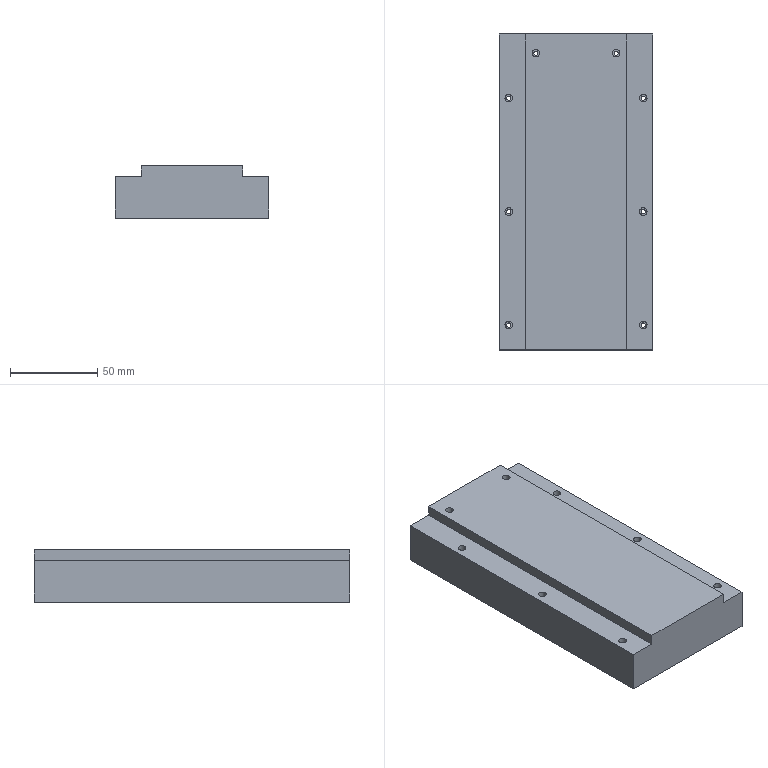NC program | NX | posted with a generic post | part box 88 x 181.05 x 30 mm
Lines 5692 to 6442 of 14572:
(CURVE_DRIVE_3_COPY , TOOL : BALL_END_R1-4-D4-50)
N11304 T14 M6
N11306 G54
N11308 G3P2 X0. Y0. Z0. I90. J12.8666 K-83.5258
N11310 G53.1
N11312 G17 G43 G0 G90 X-24.469 Y-28.966 Z32.437 S6500 H14 M3
N11314 Z2.912
N11316 G94 G1 Z1.229 F2000.
N11318 X-24.473 Z0.76
N11320 X-24.621 Y-28.979 Z0.314
N11322 X-24.898 Y-29.002 Z-0.063
N11324 X-25.279 Y-29.035 Z-0.336
N11326 X-25.725 Y-29.073 Z-0.478
N11328 X-25.965 Y-29.093 Z-0.514
N11330 X-26.205 Y-29.113 Z-0.51
N11332 X-26.462 Y-29.135 Z-0.502
N11334 X-26.833 Y-29.167 Z-0.441
N11336 X-26.956 Y-29.158
N11338 X-27.058 Y-29.143 Z-0.433
N11340 X-26.954 Y-29.134 Z-0.462
N11342 X-26.457 Y-29.092 Z-0.544
N11344 X-26.264 Y-29.075 Z-0.551
N11346 X-25.96 Y-29.05 Z-0.555
N11348 X-25.488 Y-29.009 Z-0.487
N11350 X-25.377 Y-28.961 Z-0.492
N11352 X-25.506 Y-28.972 Z-0.53
N11354 X-25.958 Y-29.01 Z-0.592
N11356 X-26.452 Y-29.052 Z-0.582
N11358 X-26.949 Y-29.095 Z-0.5
N11360 X-27.209 Y-29.117 Z-0.424
N11362 X-27.347 Y-29.087 Z-0.422
N11364 X-26.944 Y-29.052 Z-0.54
N11366 X-26.447 Y-29.01 Z-0.624
N11368 X-25.95 Y-28.968 Z-0.634
N11370 X-25.521 Y-28.931 Z-0.575
N11372 X-25.454 Y-28.926 Z-0.558
N11374 X-25.262 Y-28.909 Z-0.497
N11376 X-25.148 Y-28.858 Z-0.502
N11378 X-25.449 Y-28.884 Z-0.599
N11380 X-25.536 Y-28.891 Z-0.62
N11382 X-25.946 Y-28.926 Z-0.675
N11384 X-25.987 Y-28.929 Z-0.678
N11386 X-26.443 Y-28.968 Z-0.665
N11388 X-26.94 Y-29.01 Z-0.58
N11390 X-27.477 Y-29.056 Z-0.419
N11392 X-27.602 Y-29.025 Z-0.414
N11394 X-27.432 Y-29.01 Z-0.471
N11396 X-26.935 Y-28.968 Z-0.62
N11398 X-26.419 Y-28.924 Z-0.708
N11400 X-26.002 Y-28.889 Z-0.72
N11402 X-25.866 Y-28.877 Z-0.709
N11404 X-25.55 Y-28.85 Z-0.665
N11406 X-25.444 Y-28.841 Z-0.639
N11408 X-25.047 Y-28.808 Z-0.512
N11410 X-24.961 Y-28.76 Z-0.516
N11412 X-25.048 Y-28.768 Z-0.553
N11414 X-25.439 Y-28.801 Z-0.677
N11416 X-25.565 Y-28.812 Z-0.709
N11418 X-25.839 Y-28.835 Z-0.747
N11420 X-26.016 Y-28.85 Z-0.761
N11422 X-26.391 Y-28.882 Z-0.75
N11424 X-26.468 Y-28.888 Z-0.741
N11426 X-26.93 Y-28.928 Z-0.659
N11428 X-27.427 Y-28.97 Z-0.507
N11430 X-27.708 Y-28.994 Z-0.413
N11432 X-27.809 Y-28.962
N11434 X-27.422 Y-28.929 Z-0.545
N11436 X-26.916 Y-28.886 Z-0.701
N11438 X-26.429 Y-28.844 Z-0.787
N11440 X-26.363 Y-28.839 Z-0.793
N11442 X-26.031 Y-28.81 Z-0.803
N11444 X-25.81 Y-28.792 Z-0.785
N11446 X-25.579 Y-28.772 Z-0.753
N11448 X-25.435 Y-28.76 Z-0.717
N11450 X-25.079 Y-28.729 Z-0.604
N11452 X-24.882 Y-28.713 Z-0.517
N11454 X-24.802 Y-28.664 Z-0.518
N11456 X-24.933 Y-28.675 Z-0.581
N11458 X-25.11 Y-28.69 Z-0.656
N11460 X-25.43 Y-28.717 Z-0.757
N11462 X-25.594 Y-28.731 Z-0.798
N11464 X-25.782 Y-28.747 Z-0.824
N11466 X-26.046 Y-28.77 Z-0.846
N11468 X-26.334 Y-28.794 Z-0.837
N11470 X-26.497 Y-28.808 Z-0.817
N11472 X-26.886 Y-28.841 Z-0.748
N11474 X-27.418 Y-28.887 Z-0.583
N11476 X-27.911 Y-28.929 Z-0.413
N11478 X-28.013 Y-28.895
N11480 X-27.406 Y-28.844 Z-0.623
N11482 X-26.858 Y-28.797 Z-0.794
N11484 X-26.419 Y-28.76 Z-0.87
N11486 X-26.305 Y-28.75 Z-0.881
N11488 X-26.06 Y-28.729 Z-0.889
N11490 X-25.753 Y-28.703 Z-0.863
N11492 X-25.609 Y-28.691 Z-0.843
N11494 X-25.425 Y-28.675 Z-0.797
N11496 X-25.141 Y-28.651 Z-0.708
N11498 X-24.934 Y-28.634 Z-0.621
N11500 X-24.722 Y-28.616 Z-0.518
N11502 X-24.659 Y-28.568 Z-0.519
N11504 X-24.72 Y-28.574 Z-0.556
N11506 X-24.965 Y-28.594 Z-0.674
N11508 X-25.173 Y-28.612 Z-0.76
N11510 X-25.423 Y-28.633 Z-0.838
N11512 X-25.624 Y-28.65 Z-0.888
N11514 X-25.724 Y-28.659 Z-0.902
N11516 X-26.075 Y-28.689 Z-0.931
N11518 X-26.276 Y-28.706 Z-0.925
N11520 X-26.414 Y-28.718 Z-0.912
N11522 X-26.829 Y-28.753 Z-0.84
N11524 X-26.911 Y-28.76 Z-0.818
N11526 X-27.347 Y-28.797 Z-0.68
N11528 X-28.115 Y-28.862 Z-0.412
N11530 X-28.217 Y-28.829
N11532 X-27.289 Y-28.75 Z-0.737
N11534 X-26.906 Y-28.718 Z-0.858
N11536 X-26.8 Y-28.709 Z-0.887
N11538 X-26.409 Y-28.676 Z-0.954
N11540 X-26.248 Y-28.662 Z-0.969
N11542 X-26.09 Y-28.648 Z-0.974
N11544 X-25.695 Y-28.615 Z-0.941
N11546 X-25.638 Y-28.61 Z-0.933
N11548 X-25.416 Y-28.591 Z-0.878
N11550 X-25.187 Y-28.572 Z-0.807
N11552 X-24.919 Y-28.549 Z-0.692
N11554 X-24.735 Y-28.533 Z-0.603
N11556 X-24.601 Y-28.522 Z-0.522
N11558 X-24.546 Y-28.475 Z-0.526
N11560 X-24.75 Y-28.493 Z-0.649
N11562 X-25.028 Y-28.516 Z-0.781
N11564 X-25.235 Y-28.534 Z-0.865
N11566 X-25.411 Y-28.549 Z-0.919
N11568 X-25.666 Y-28.571 Z-0.98
N11570 X-26.105 Y-28.608 Z-1.017
N11572 X-26.219 Y-28.618 Z-1.013
N11574 X-26.405 Y-28.633 Z-0.995
N11576 X-26.771 Y-28.664 Z-0.933
N11578 X-26.902 Y-28.676 Z-0.898
N11580 X-27.23 Y-28.704 Z-0.794
N11582 X-28.32 Y-28.796 Z-0.412
N11584 X-28.424 Y-28.763
N11586 X-28.282 Y-28.751 Z-0.459
N11588 X-27.171 Y-28.657 Z-0.851
N11590 X-26.897 Y-28.633 Z-0.938
N11592 X-26.742 Y-28.62 Z-0.98
N11594 X-26.4 Y-28.591 Z-1.037
N11596 X-26.19 Y-28.573 Z-1.057
N11598 X-26.12 Y-28.567 Z-1.06
N11600 X-25.668 Y-28.529 Z-1.023
N11602 X-25.406 Y-28.507 Z-0.961
N11604 X-25.217 Y-28.49 Z-0.9
N11606 X-25.059 Y-28.477 Z-0.835
N11608 X-24.765 Y-28.452 Z-0.696
N11610 X-24.492 Y-28.429 Z-0.531
N11612 X-24.441 Y-28.383 Z-0.534
N11614 X-24.78 Y-28.412 Z-0.741
N11616 X-25.09 Y-28.438 Z-0.888
N11618 X-25.297 Y-28.456 Z-0.97
N11620 X-25.401 Y-28.465 Z-1.002
N11622 X-25.683 Y-28.489 Z-1.068
N11624 X-26.134 Y-28.527 Z-1.102
N11626 X-26.395 Y-28.549 Z-1.078
N11628 X-26.714 Y-28.576 Z-1.026
N11630 X-26.892 Y-28.592 Z-0.978
N11632 X-27.113 Y-28.61 Z-0.908
N11634 X-28.523 Y-28.73 Z-0.411
N11636 X-28.625 Y-28.698
N11638 X-27.054 Y-28.564 Z-0.964
N11640 X-26.887 Y-28.55 Z-1.017
N11642 X-26.685 Y-28.533 Z-1.072
N11644 X-26.39 Y-28.508 Z-1.12
N11646 X-26.133 Y-28.486 Z-1.144
N11648 X-25.741 Y-28.452 Z-1.116
N11650 X-25.645 Y-28.444 Z-1.103
N11652 X-25.397 Y-28.423 Z-1.043
N11654 X-25.246 Y-28.41 Z-0.992
N11656 X-25.121 Y-28.4 Z-0.94
N11658 X-24.794 Y-28.372 Z-0.787
N11660 X-24.569 Y-28.353 Z-0.652
N11662 X-24.391 Y-28.337 Z-0.536
N11664 X-24.343 Y-28.292 Z-0.537
N11666 X-24.625 Y-28.316 Z-0.723
N11668 X-24.809 Y-28.332 Z-0.833
N11670 X-25.151 Y-28.361 Z-0.993
N11672 X-25.358 Y-28.378 Z-1.074
N11674 X-25.64 Y-28.402 Z-1.144
N11676 X-25.772 Y-28.414 Z-1.162
N11678 X-26.137 Y-28.445 Z-1.186
N11680 X-26.43 Y-28.47 Z-1.154
N11682 X-26.657 Y-28.489 Z-1.118
N11684 X-26.883 Y-28.508 Z-1.057
N11686 X-26.996 Y-28.518 Z-1.021
N11688 X-28.727 Y-28.665 Z-0.411
N11690 X-28.83 Y-28.632 Z-0.412
N11692 X-26.878 Y-28.466 Z-1.096
N11694 X-26.629 Y-28.445 Z-1.164
N11696 X-26.381 Y-28.424 Z-1.204
N11698 X-26.132 Y-28.403 Z-1.228
N11700 X-25.803 Y-28.375 Z-1.208
N11702 X-25.727 Y-28.368 Z-1.201
N11704 X-25.635 Y-28.36 Z-1.185
N11706 X-25.389 Y-28.34 Z-1.127
N11708 X-25.182 Y-28.322 Z-1.046
N11710 X-24.824 Y-28.291 Z-0.879
N11712 X-24.682 Y-28.279 Z-0.794
N11714 X-24.393 Y-28.255 Z-0.607
N11716 X-24.294 Y-28.246 Z-0.539
N11718 X-24.247 Y-28.201
N11720 X-24.388 Y-28.213 Z-0.639
N11722 X-24.738 Y-28.243 Z-0.865
N11724 X-24.838 Y-28.251 Z-0.925
N11726 X-25.213 Y-28.283 Z-1.099
N11728 X-25.382 Y-28.297 Z-1.165
N11730 X-25.631 Y-28.319 Z-1.226
N11732 X-25.742 Y-28.328 Z-1.245
N11734 X-25.947 Y-28.346 Z-1.262
N11736 X-26.128 Y-28.361 Z-1.27
N11738 X-26.376 Y-28.382 Z-1.247
N11740 X-26.6 Y-28.401 Z-1.211
N11742 X-26.879 Y-28.425 Z-1.134
N11744 X-28.932 Y-28.599 Z-0.411
N11746 X-29.033 Y-28.567
N11748 X-26.868 Y-28.382 Z-1.175
N11750 X-26.571 Y-28.357 Z-1.258
N11752 X-26.371 Y-28.34 Z-1.29
N11754 X-26.123 Y-28.319 Z-1.312
N11756 X-25.874 Y-28.298 Z-1.301
N11758 X-25.756 Y-28.288 Z-1.29
N11760 X-25.626 Y-28.277 Z-1.267
N11762 X-25.451 Y-28.262 Z-1.226
N11764 X-25.378 Y-28.256 Z-1.204
N11766 X-25.244 Y-28.244 Z-1.152
N11768 X-24.853 Y-28.211 Z-0.971
N11770 X-24.416 Y-28.174 Z-0.694
N11772 X-24.202 Y-28.156 Z-0.541
N11774 X-24.163 Y-28.111
N11776 X-24.191 Y-28.113 Z-0.565
N11778 X-24.379 Y-28.129 Z-0.698
N11780 X-24.448 Y-28.135 Z-0.751
N11782 X-24.868 Y-28.171 Z-1.018
N11784 X-25.32 Y-28.209 Z-1.224
N11786 X-25.373 Y-28.214 Z-1.243
N11788 X-25.482 Y-28.223 Z-1.275
N11790 X-25.621 Y-28.235 Z-1.308
N11792 X-25.771 Y-28.248 Z-1.334
N11794 X-25.87 Y-28.256 Z-1.344
N11796 X-26.118 Y-28.277 Z-1.355
N11798 X-26.367 Y-28.298 Z-1.333
N11800 X-26.542 Y-28.313 Z-1.304
N11802 X-26.864 Y-28.34 Z-1.214
N11804 X-29.137 Y-28.534 Z-0.412
N11806 X-29.241 Y-28.501 Z-0.413
N11808 X-29.163 Y-28.494 Z-0.437
N11810 X-26.859 Y-28.298 Z-1.253
N11812 X-26.514 Y-28.269 Z-1.351
N11814 X-26.362 Y-28.256 Z-1.376
N11816 X-26.113 Y-28.235 Z-1.397
N11818 X-25.865 Y-28.214 Z-1.387
N11820 X-25.786 Y-28.207 Z-1.379
N11822 X-25.616 Y-28.193 Z-1.35
N11824 X-25.513 Y-28.184 Z-1.325
N11826 X-25.334 Y-28.169 Z-1.27
N11828 X-24.883 Y-28.13 Z-1.064
N11830 X-24.479 Y-28.096 Z-0.808
N11832 X-24.374 Y-28.087 Z-0.728
N11834 X-24.205 Y-28.073 Z-0.609
N11836 X-24.127 Y-28.066 Z-0.54
N11838 X-24.091 Y-28.021 Z-0.538
N11840 X-24.22 Y-28.032 Z-0.652
N11842 X-24.369 Y-28.045 Z-0.758
N11844 X-24.51 Y-28.057 Z-0.866
N11846 X-24.898 Y-28.09 Z-1.111
N11848 X-25.363 Y-28.13 Z-1.322
N11850 X-25.544 Y-28.145 Z-1.375
N11852 X-25.612 Y-28.151 Z-1.391
N11854 X-25.801 Y-28.167 Z-1.424
N11856 X-25.933 Y-28.178 Z-1.433
N11858 X-26.109 Y-28.193 Z-1.439
N11860 X-26.357 Y-28.214 Z-1.419
N11862 X-26.485 Y-28.225 Z-1.398
N11864 X-26.854 Y-28.256 Z-1.292
N11866 X-28.648 Y-28.409 Z-0.654
N11868 X-29.22 Y-28.458 Z-0.453
N11870 X-29.346 Y-28.468 Z-0.414
N11872 X-29.447 Y-28.435 Z-0.413
N11874 X-29.276 Y-28.421 Z-0.469
N11876 X-27.346 Y-28.257 Z-1.153
N11878 X-26.849 Y-28.214 Z-1.332
N11880 X-26.456 Y-28.181 Z-1.445
N11882 X-26.352 Y-28.172 Z-1.462
N11884 X-26.104 Y-28.151 Z-1.482
N11886 X-25.816 Y-28.126 Z-1.468
N11888 X-25.575 Y-28.106 Z-1.425
N11890 X-25.352 Y-28.087 Z-1.358
N11892 X-24.912 Y-28.05 Z-1.158
N11894 X-24.541 Y-28.018 Z-0.923
N11896 X-24.365 Y-28.003 Z-0.787
N11898 X-24.235 Y-27.992 Z-0.696
N11900 X-24.056 Y-27.977 Z-0.538
N11902 X-24.023 Y-27.933 Z-0.539
N11904 X-24.25 Y-27.952 Z-0.739
N11906 X-24.36 Y-27.961 Z-0.816
N11908 X-24.572 Y-27.979 Z-0.98
N11910 X-24.927 Y-28.01 Z-1.205
N11912 X-25.354 Y-28.046 Z-1.401
N11914 X-25.432 Y-28.052 Z-1.427
N11916 X-25.613 Y-28.068 Z-1.475
N11918 X-25.851 Y-28.088 Z-1.514
N11920 X-26.099 Y-28.109 Z-1.523
N11922 X-26.348 Y-28.13 Z-1.505
N11924 X-26.428 Y-28.137 Z-1.492
N11926 X-26.529 Y-28.146 Z-1.464
N11928 X-26.606 Y-28.152 Z-1.447
N11930 X-26.851 Y-28.173 Z-1.368
N11932 X-27.469 Y-28.226 Z-1.144
N11934 X-29.546 Y-28.402 Z-0.412
N11936 X-29.64 Y-28.372 Z-0.411
N11938 X-27.498 Y-28.189 Z-1.167
N11940 X-26.877 Y-28.136 Z-1.395
N11942 X-26.857 Y-28.135 Z-1.404
N11944 X-26.946 Y-28.105 Z-1.402
N11946 X-27.526 Y-28.154 Z-1.19
N11948 X-29.731 Y-28.342 Z-0.41
N11950 X-29.824 Y-28.312
N11952 X-27.555 Y-28.119 Z-1.213
N11954 X-27.038 Y-28.075 Z-1.402
N11956 X-27.137 Y-28.042 Z-1.403
N11958 X-27.585 Y-28.081 Z-1.237
N11960 X-29.927 Y-28.28 Z-0.411
N11962 X-30.035 Y-28.246 Z-0.413
N11964 X-29.803 Y-28.226 Z-0.491
N11966 X-27.618 Y-28.04 Z-1.263
N11968 X-27.24 Y-28.008 Z-1.404
N11970 X-27.343 Y-27.974
N11972 X-27.65 Y-28. Z-1.29
N11974 X-29.798 Y-28.183 Z-0.53
N11976 X-30.143 Y-28.212 Z-0.413
N11978 X-30.248 Y-28.178
N11980 X-29.793 Y-28.139 Z-0.569
N11982 X-27.682 Y-27.96 Z-1.316
N11984 X-27.444 Y-27.94 Z-1.404
N11986 X-27.547 Y-27.905
N11988 X-28.233 Y-27.964 Z-1.158
N11990 X-29.814 Y-28.098 Z-0.6
N11992 X-30.353 Y-28.144 Z-0.413
N11994 X-30.46 Y-28.109 Z-0.412
N11996 X-28.303 Y-27.926 Z-1.171
N11998 X-27.653 Y-27.87 Z-1.403
N12000 X-27.753 Y-27.838
N12002 X-30.561 Y-28.076 Z-0.412
N12004 X-30.667 Y-28.042 Z-0.411
N12006 X-27.861 Y-27.803 Z-1.403
N12008 X-27.972 Y-27.769 Z-1.404
N12010 X-28.144 Y-27.783 Z-1.34
N12012 X-30.722 Y-28.003 Z-0.429
N12014 X-30.777 Y-28.007 Z-0.412
N12016 X-30.886 Y-27.971 Z-0.411
N12018 X-28.297 Y-27.751 Z-1.326
N12020 X-28.086 Y-27.733 Z-1.405
N12022 X-28.199 Y-27.698 Z-1.406
N12024 X-28.599 Y-27.732 Z-1.258
N12026 X-30.997 Y-27.936 Z-0.411
N12028 X-31.108 Y-27.9
N12030 X-28.715 Y-27.696 Z-1.258
N12032 X-28.311 Y-27.662 Z-1.407
N12034 X-28.424 Y-27.627 Z-1.408
N12036 X-28.839 Y-27.662 Z-1.251
N12038 X-31.219 Y-27.865 Z-0.411
N12040 X-31.329 Y-27.829
N12042 X-28.749 Y-27.61 Z-1.323
N12044 X-28.533 Y-27.591 Z-1.407
N12046 X-28.639 Y-27.555 Z-1.405
N12048 X-28.962 Y-27.583 Z-1.286
N12050 X-31.44 Y-27.794 Z-0.411
N12052 X-31.551 Y-27.759 Z-0.412
N12054 X-29.022 Y-27.544 Z-1.303
N12056 X-28.743 Y-27.52 Z-1.403
N12058 X-28.85 Y-27.486
N12060 X-31.563 Y-27.716 Z-0.443
N12062 X-31.66 Y-27.725 Z-0.413
N12064 X-31.767 Y-27.69
N12066 X-31.622 Y-27.678 Z-0.459
N12068 X-28.956 Y-27.451 Z-1.403
N12070 X-29.069 Y-27.417 Z-1.404
N12072 X-29.269 Y-27.434 Z-1.33
N12074 X-31.705 Y-27.641 Z-0.469
N12076 X-31.873 Y-27.655 Z-0.412
N12078 X-31.98 Y-27.62 Z-0.411
N12080 X-29.863 Y-27.44 Z-1.158
N12082 X-29.713 Y-27.427 Z-1.214
N12084 X-29.24 Y-27.387 Z-1.381
N12086 X-29.181 Y-27.382 Z-1.405
N12088 X-29.29 Y-27.346 Z-1.404
N12090 X-30.526 Y-27.451 Z-0.963
N12092 X-32.09 Y-27.584 Z-0.41
N12094 X-32.203 Y-27.548
N12096 X-29.931 Y-27.354 Z-1.214
N12098 X-29.702 Y-27.335 Z-1.299
N12100 X-29.401 Y-27.309 Z-1.404
N12102 X-29.512 Y-27.274 Z-1.405
N12104 X-30.518 Y-27.36 Z-1.045
N12106 X-32.316 Y-27.513 Z-0.411
N12108 X-32.426 Y-27.478 Z-0.413
N12110 X-32.177 Y-27.457 Z-0.496
N12112 X-29.997 Y-27.272 Z-1.267
N12114 X-29.622 Y-27.24 Z-1.405
N12116 X-29.728 Y-27.206
N12118 X-30.029 Y-27.231 Z-1.293
N12120 X-32.172 Y-27.414 Z-0.535
N12122 X-32.533 Y-27.444 Z-0.413
N12124 X-32.639 Y-27.41
N12126 X-31.64 Y-27.325 Z-0.761
N12128 X-30.061 Y-27.191 Z-1.32
N12130 X-29.833 Y-27.171 Z-1.405
N12132 X-29.939 Y-27.136 Z-1.404
N12134 X-31.133 Y-27.238 Z-0.979
N12136 X-32.172 Y-27.326 Z-0.611
N12138 X-32.746 Y-27.375 Z-0.412
N12140 X-32.854 Y-27.34
N12142 X-30.694 Y-27.156 Z-1.173
N12144 X-30.046 Y-27.101 Z-1.403
N12146 X-30.154 Y-27.066 Z-1.402
N12148 X-32.963 Y-27.305 Z-0.411
N12150 X-33.073 Y-27.269 Z-0.412
N12152 X-30.267 Y-27.031 Z-1.403
N12154 X-30.379 Y-26.996 Z-1.405
N12156 X-30.592 Y-27.014 Z-1.325
N12158 X-33.135 Y-27.23 Z-0.427
N12160 X-33.183 Y-27.234 Z-0.412
N12162 X-33.292 Y-27.198 Z-0.411
N12164 X-30.645 Y-26.973 Z-1.348
N12166 X-30.493 Y-26.96 Z-1.406
N12168 X-30.606 Y-26.924
N12170 X-31.048 Y-26.962 Z-1.243
N12172 X-33.404 Y-27.162 Z-0.411
N12174 X-33.516 Y-27.127
N12176 X-31.132 Y-26.924 Z-1.252
N12178 X-30.718 Y-26.889 Z-1.407
N12180 X-30.83 Y-26.854 Z-1.408
N12182 X-31.234 Y-26.888 Z-1.255
N12184 X-33.626 Y-27.092 Z-0.411
N12186 X-33.736 Y-27.056
N12188 X-31.122 Y-26.834 Z-1.335
N12190 X-30.937 Y-26.818 Z-1.406
N12192 X-31.043 Y-26.782 Z-1.404
N12194 X-31.848 Y-26.851 Z-1.116
N12196 X-33.847 Y-27.021 Z-0.411
N12198 X-33.958 Y-26.986 Z-0.412
N12200 X-32.602 Y-26.871 Z-0.888
N12202 X-31.148 Y-26.747 Z-1.403
N12204 X-31.254 Y-26.713
N12206 X-33.957 Y-26.943 Z-0.447
N12208 X-34.066 Y-26.952 Z-0.413
N12210 X-34.172 Y-26.917
N12212 X-34.016 Y-26.904 Z-0.463
N12214 X-31.362 Y-26.678 Z-1.403
N12216 X-31.477 Y-26.644 Z-1.405
N12218 X-31.595 Y-26.654 Z-1.358
N12220 X-34.078 Y-26.865 Z-0.48
N12222 X-34.279 Y-26.882 Z-0.412
N12224 X-34.387 Y-26.847 Z-0.411
N12226 X-32.248 Y-26.665 Z-1.166
N12228 X-32.085 Y-26.651 Z-1.226
N12230 X-31.618 Y-26.611 Z-1.392
N12232 X-31.588 Y-26.609 Z-1.406
N12234 X-31.696 Y-26.572 Z-1.404
N12236 X-34.068 Y-26.774 Z-0.562
N12238 X-34.498 Y-26.81 Z-0.41
N12240 X-34.611 Y-26.775 Z-0.411
N12242 X-32.316 Y-26.579 Z-1.221
N12244 X-32.075 Y-26.559 Z-1.311
N12246 X-31.807 Y-26.536 Z-1.404
N12248 X-31.918 Y-26.501 Z-1.405
N12250 X-32.9 Y-26.585 Z-1.053
N12252 X-34.554 Y-26.726 Z-0.468
N12254 X-34.723 Y-26.74 Z-0.412
N12256 X-34.832 Y-26.706 Z-0.413
N12258 X-34.549 Y-26.682 Z-0.508
N12260 X-32.381 Y-26.497 Z-1.274
N12262 X-32.027 Y-26.467 Z-1.406
N12264 X-32.132 Y-26.433 Z-1.405
N12266 X-32.414 Y-26.457 Z-1.3
N12268 X-34.544 Y-26.638 Z-0.547
N12270 X-34.939 Y-26.672 Z-0.413
N12272 X-35.045 Y-26.637
N12274 X-34.016 Y-26.55 Z-0.772
N12276 X-32.446 Y-26.416 Z-1.327
N12278 X-32.238 Y-26.398 Z-1.405
N12280 X-32.344 Y-26.363 Z-1.404
N12282 X-34.619 Y-26.557 Z-0.597
N12284 X-35.152 Y-26.602 Z-0.412
N12286 X-35.26 Y-26.567
N12288 X-32.512 Y-26.333 Z-1.38
N12290 X-32.452 Y-26.328 Z-1.403
N12292 X-32.561 Y-26.293
N12294 X-35.37 Y-26.532 Z-0.411
N12296 X-35.48 Y-26.497 Z-0.412
N12298 X-34.673 Y-26.428 Z-0.694
N12300 X-32.815 Y-26.27 Z-1.351
N12302 X-32.674 Y-26.258 Z-1.404
N12304 X-32.787 Y-26.223 Z-1.405
N12306 X-33.041 Y-26.244 Z-1.31
N12308 X-35.589 Y-26.461 Z-0.411
N12310 X-35.7 Y-26.425
N12312 X-33.27 Y-26.218 Z-1.269
N12314 X-32.9 Y-26.187 Z-1.406
N12316 X-33.012 Y-26.151
N12318 X-33.51 Y-26.194 Z-1.223
N12320 X-35.811 Y-26.389 Z-0.411
N12322 X-35.922 Y-26.354
N12324 X-33.505 Y-26.148 Z-1.264
N12326 X-33.125 Y-26.116 Z-1.407
N12328 X-33.236 Y-26.081 Z-1.408
N12330 X-33.628 Y-26.114 Z-1.259
N12332 X-36.033 Y-26.319 Z-0.411
N12334 X-36.143 Y-26.283
N12336 X-33.494 Y-26.058 Z-1.347
N12338 X-33.342 Y-26.045 Z-1.406
N12340 X-33.447 Y-26.009 Z-1.404
N12342 X-36.232 Y-26.246 Z-0.418
N12344 X-36.254 Y-26.248 Z-0.411
N12346 X-36.364 Y-26.213 Z-0.412
N12348 X-36.292 Y-26.207 Z-0.434
N12350 X-33.553 Y-25.974 Z-1.403
N12352 X-33.659 Y-25.94
N12354 X-36.35 Y-26.169 Z-0.451
N12356 X-36.471 Y-26.179 Z-0.413
N12358 X-36.577 Y-26.145 Z-0.412
N12360 X-36.41 Y-26.13 Z-0.467
N12362 X-33.769 Y-25.906 Z-1.404
N12364 X-33.883 Y-25.871 Z-1.405
N12366 X-33.988 Y-25.88 Z-1.363
N12368 X-36.685 Y-26.109 Z-0.411
N12370 X-36.793 Y-26.074 Z-0.41
N12372 X-34.633 Y-25.89 Z-1.173
N12374 X-34.458 Y-25.875 Z-1.238
N12376 X-34.049 Y-25.84 Z-1.381
N12378 X-33.994 Y-25.835 Z-1.405
N12380 X-34.102 Y-25.799 Z-1.404
N12382 X-34.453 Y-25.829 Z-1.281
N12384 X-34.667 Y-25.847 Z-1.201
N12386 X-36.905 Y-26.037 Z-0.41
N12388 X-37.018 Y-26.002 Z-0.411
N12390 X-34.701 Y-25.805 Z-1.228
N12392 X-34.447 Y-25.783 Z-1.323
N12394 X-34.214 Y-25.763 Z-1.404
N12396 X-34.323 Y-25.729 Z-1.405
N12398 X-34.734 Y-25.763 Z-1.255
N12400 X-36.927 Y-25.95 Z-0.48
N12402 X-37.129 Y-25.967 Z-0.412
N12404 X-37.238 Y-25.933 Z-0.413
N12406 X-36.922 Y-25.907 Z-0.519
N12408 X-34.766 Y-25.723 Z-1.281
N12410 X-34.431 Y-25.695 Z-1.406
N12412 X-34.536 Y-25.66 Z-1.405
N12414 X-34.798 Y-25.683 Z-1.307
N12416 X-36.917 Y-25.863 Z-0.558
N12418 X-37.343 Y-25.899 Z-0.413
N12420 X-37.45 Y-25.865 Z-0.412
N12422 X-36.392 Y-25.775 Z-0.782
N12424 X-34.831 Y-25.642 Z-1.334
N12426 X-34.641 Y-25.626 Z-1.404
N12428 X-34.748 Y-25.591
N12430 X-37.064 Y-25.788 Z-0.583
N12432 X-37.557 Y-25.83 Z-0.412
N12434 X-37.666 Y-25.794 Z-0.411
N12436 X-34.856 Y-25.555 Z-1.403
N12438 X-34.968 Y-25.52
N12440 X-37.775 Y-25.759 Z-0.411
N12442 X-37.886 Y-25.724 Z-0.412
N12444 X-37.738 Y-25.711 Z-0.461
N12446 X-35.261 Y-25.501 Z-1.336
N12448 X-35.079 Y-25.485 Z-1.404
N12450 X-35.193 Y-25.45 Z-1.405
N12452 X-35.489 Y-25.475 Z-1.295
N12454 X-37.995 Y-25.688 Z-0.411
N12456 X-38.106 Y-25.652
N12458 X-35.717 Y-25.449 Z-1.254
N12460 X-35.306 Y-25.414 Z-1.406
N12462 X-35.418 Y-25.378 Z-1.407
N12464 X-35.882 Y-25.418 Z-1.235
N12466 X-38.218 Y-25.617 Z-0.411
N12468 X-38.328 Y-25.581
N12470 X-35.877 Y-25.373 Z-1.276
N12472 X-35.53 Y-25.343 Z-1.407
N12474 X-35.64 Y-25.308
N12476 X-35.872 Y-25.328 Z-1.317
N12478 X-38.438 Y-25.546 Z-0.411
N12480 X-38.549 Y-25.51
N12482 X-35.867 Y-25.282 Z-1.358
N12484 X-35.746 Y-25.272 Z-1.405
N12486 X-35.85 Y-25.236 Z-1.403
N12488 X-38.626 Y-25.472 Z-0.422
N12490 X-38.659 Y-25.475 Z-0.411
N12492 X-38.769 Y-25.441 Z-0.412
N12494 X-38.685 Y-25.434 Z-0.438
N12496 X-35.957 Y-25.202 Z-1.403
N12498 X-36.063 Y-25.167
N12500 X-38.744 Y-25.396 Z-0.455
N12502 X-38.876 Y-25.407 Z-0.413
N12504 X-38.983 Y-25.372 Z-0.412
N12506 X-38.804 Y-25.356 Z-0.471
N12508 X-36.266 Y-25.141 Z-1.369
N12510 X-36.176 Y-25.133 Z-1.404
N12512 X-36.288 Y-25.098 Z-1.406
N12514 X-36.382 Y-25.106 Z-1.367
N12516 X-39.089 Y-25.337 Z-0.411
N12518 X-39.198 Y-25.301 Z-0.41
N12520 X-37.018 Y-25.115 Z-1.18
N12522 X-36.83 Y-25.099 Z-1.25
N12524 X-36.443 Y-25.067 Z-1.385
N12526 X-36.397 Y-25.063 Z-1.405
N12528 X-36.506 Y-25.026 Z-1.404
N12530 X-36.825 Y-25.053 Z-1.292
N12532 X-37.052 Y-25.073 Z-1.208
N12534 X-39.311 Y-25.265 Z-0.41
N12536 X-39.424 Y-25.229 Z-0.411
N12538 X-37.086 Y-25.031 Z-1.235
N12540 X-36.618 Y-24.991 Z-1.404
N12542 X-36.727 Y-24.956 Z-1.405
N12544 X-37.118 Y-24.99 Z-1.262
N12546 X-39.3 Y-25.175 Z-0.49
N12548 X-39.534 Y-25.195 Z-0.412
N12550 X-39.641 Y-25.161 Z-0.413
N12552 X-39.295 Y-25.132 Z-0.53
N12554 X-37.15 Y-24.95 Z-1.288
N12556 X-36.833 Y-24.923 Z-1.405
N12558 X-36.938 Y-24.888
N12560 X-37.183 Y-24.909 Z-1.314
N12562 X-39.29 Y-25.088 Z-0.569
N12564 X-39.747 Y-25.127 Z-0.413
N12566 X-39.853 Y-25.092 Z-0.412
N12568 X-38.768 Y-25. Z-0.792
N12570 X-37.215 Y-24.868 Z-1.341
N12572 X-37.044 Y-24.853 Z-1.404
N12574 X-37.151 Y-24.818 Z-1.403
N12576 X-39.507 Y-25.019 Z-0.569
N12578 X-39.961 Y-25.057 Z-0.412
N12580 X-40.07 Y-25.022 Z-0.411
N12582 X-37.26 Y-24.783 Z-1.403
N12584 X-37.373 Y-24.747 Z-1.404
N12586 X-40.18 Y-24.986 Z-0.411
N12588 X-40.291 Y-24.951
N12590 X-39.564 Y-24.889 Z-0.665
N12592 X-37.707 Y-24.731 Z-1.322
N12594 X-37.485 Y-24.712 Z-1.405
N12596 X-37.599 Y-24.677 Z-1.406
N12598 X-37.936 Y-24.705 Z-1.281
N12600 X-40.4 Y-24.915 Z-0.41
N12602 X-40.512 Y-24.879
N12604 X-38.163 Y-24.679 Z-1.24
N12606 X-37.712 Y-24.641 Z-1.406
N12608 X-37.824 Y-24.606 Z-1.407
N12610 X-38.255 Y-24.642 Z-1.246
N12612 X-40.624 Y-24.844 Z-0.411
N12614 X-40.734 Y-24.809
N12616 X-38.25 Y-24.597 Z-1.287
N12618 X-37.935 Y-24.571 Z-1.408
N12620 X-38.043 Y-24.535 Z-1.407
N12622 X-38.245 Y-24.552 Z-1.328
N12624 X-40.844 Y-24.773 Z-0.411
N12626 X-40.954 Y-24.738
N12628 X-38.24 Y-24.507 Z-1.37
N12630 X-38.149 Y-24.499 Z-1.405
N12632 X-38.254 Y-24.464 Z-1.403
N12634 X-41.019 Y-24.699 Z-0.426
N12636 X-41.065 Y-24.703 Z-0.412
N12638 X-41.174 Y-24.669 Z-0.413
N12640 X-41.081 Y-24.661 Z-0.441
N12642 X-38.36 Y-24.429 Z-1.403
N12644 X-38.468 Y-24.395
N12646 X-41.139 Y-24.622 Z-0.458
N12648 X-41.28 Y-24.634 Z-0.412
N12650 X-41.387 Y-24.599 Z-0.411
N12652 X-39.957 Y-24.477 Z-0.914
N12654 X-38.716 Y-24.372 Z-1.353
N12656 X-38.583 Y-24.36 Z-1.405
N12658 X-38.695 Y-24.325 Z-1.406
N12660 X-38.776 Y-24.332 Z-1.371
N12662 X-41.495 Y-24.564 Z-0.41
N12664 X-41.605 Y-24.528
N12666 X-39.404 Y-24.34 Z-1.188
N12668 X-39.203 Y-24.323 Z-1.262
N12670 X-38.837 Y-24.292 Z-1.39
N12672 X-38.803 Y-24.289 Z-1.405
N12674 X-38.913 Y-24.253 Z-1.404
N12676 X-39.198 Y-24.277 Z-1.304
N12678 X-39.438 Y-24.298 Z-1.216
N12680 X-41.718 Y-24.492 Z-0.41
N12682 X-41.83 Y-24.457 Z-0.411
N12684 X-40.574 Y-24.35 Z-0.852
N12686 X-39.471 Y-24.256 Z-1.242
N12688 X-39.023 Y-24.218 Z-1.405
N12690 X-39.131 Y-24.184
N12692 X-39.503 Y-24.216 Z-1.269
N12694 X-41.672 Y-24.4 Z-0.502
N12696 X-41.94 Y-24.423 Z-0.412
N12698 X-42.046 Y-24.389 Z-0.413
N12700 X-41.667 Y-24.357 Z-0.541
N12702 X-39.535 Y-24.175 Z-1.295
N12704 X-39.237 Y-24.15 Z-1.405
N12706 X-39.342 Y-24.115
N12708 X-40.091 Y-24.179 Z-1.136
N12710 X-41.765 Y-24.322 Z-0.546
N12712 X-42.152 Y-24.354 Z-0.412
N12714 X-42.259 Y-24.32
N12716 X-41.198 Y-24.229 Z-0.783
N12718 X-39.449 Y-24.081 Z-1.404
N12720 X-39.556 Y-24.045 Z-1.403
N12722 X-41.954 Y-24.249 Z-0.554
N12724 X-42.367 Y-24.284 Z-0.411
N12726 X-42.476 Y-24.249
N12728 X-39.666 Y-24.01 Z-1.403
N12730 X-39.779 Y-23.975 Z-1.404
N12732 X-42.405 Y-24.198 Z-0.472
N12734 X-42.586 Y-24.214 Z-0.411
N12736 X-42.696 Y-24.178
N12738 X-40.155 Y-23.962 Z-1.307
N12740 X-39.892 Y-23.939 Z-1.405
N12742 X-40.005 Y-23.904 Z-1.406
N12744 X-40.383 Y-23.936 Z-1.266
N12746 X-42.807 Y-24.142 Z-0.41
N12748 X-42.919 Y-24.106
N12750 X-40.61 Y-23.91 Z-1.225
N12752 X-40.117 Y-23.868 Z-1.406
N12754 X-40.229 Y-23.833 Z-1.407
N12756 X-40.628 Y-23.867 Z-1.258
N12758 X-43.03 Y-24.071 Z-0.411
N12760 X-43.14 Y-24.036
N12762 X-40.622 Y-23.822 Z-1.299
N12764 X-40.341 Y-23.798 Z-1.408
N12766 X-40.446 Y-23.762 Z-1.406
N12768 X-40.809 Y-23.793 Z-1.271
N12770 X-43.249 Y-24. Z-0.411
N12772 X-43.36 Y-23.965
N12774 X-40.612 Y-23.731 Z-1.381
N12776 X-40.552 Y-23.726 Z-1.404
N12778 X-40.658 Y-23.691 Z-1.403
N12780 X-43.412 Y-23.925 Z-0.429
N12782 X-43.47 Y-23.93 Z-0.412
N12784 X-43.579 Y-23.897 Z-0.413
N12786 X-43.471 Y-23.887 Z-0.446
N12788 X-40.764 Y-23.657 Z-1.403
N12790 X-40.874 Y-23.623 Z-1.404
N12792 X-43.53 Y-23.849 Z-0.462
N12794 X-43.684 Y-23.862 Z-0.412
N12796 X-43.791 Y-23.827 Z-0.411
N12798 X-41.089 Y-23.597 Z-1.366